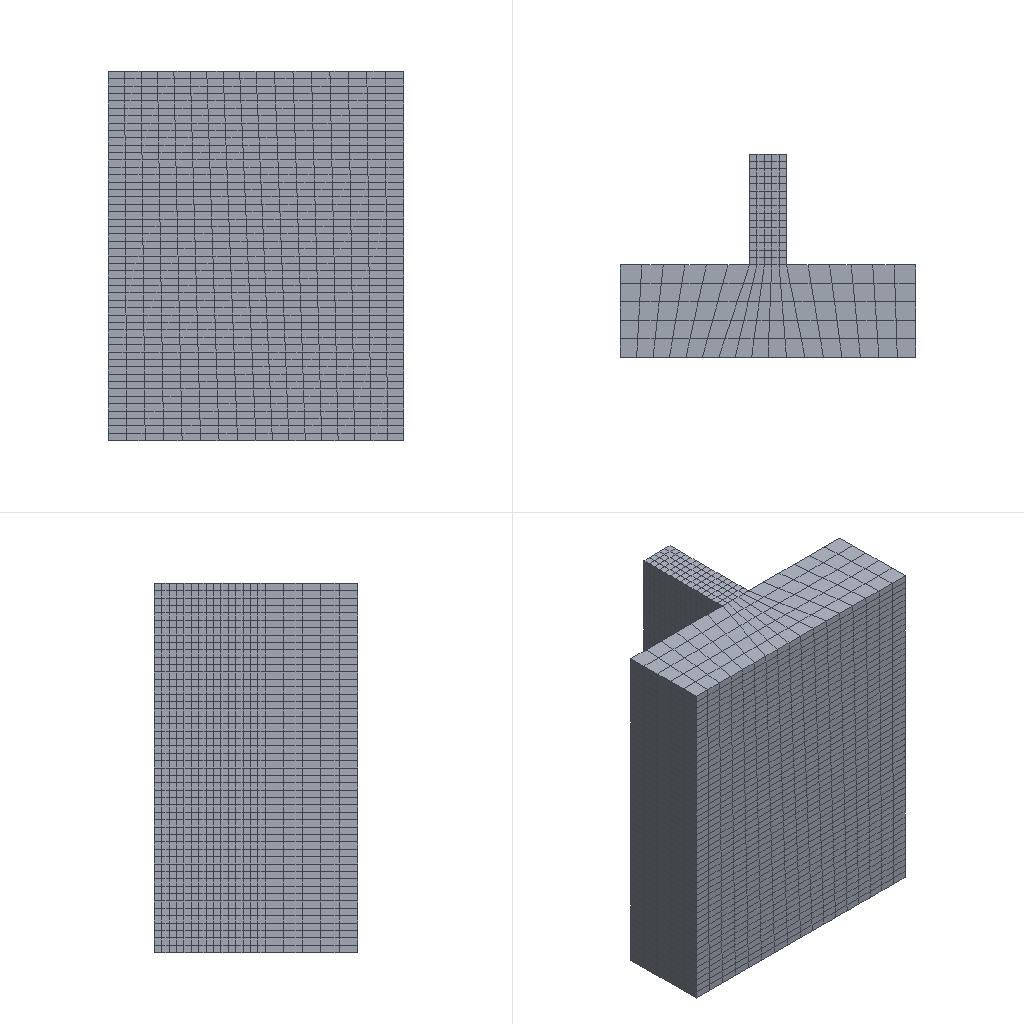Simulation study | abaqus
Set-up summary:
category,name,step,type,value,unit,region
solver,abaqus
solver,version,,,Abaqus/Standard 3DEXPERIENCE R2017x
units,not stated in the deck,,not stated
analysis,deck,,thermal,thermal
load_step,Step-kill,Step-kill,thermal
load_step,add-1,add-1,thermal
load_step,add-2,add-2,thermal
load_step,add-3,add-3,thermal
load_step,add-4,add-4,thermal
load_step,add-5,add-5,thermal
load_step,add-6,add-6,thermal
load_step,add-7,add-7,thermal
load_step,add-8,add-8,thermal
load_step,add-9,add-9,thermal
load_step,add-10,add-10,thermal
load_step,add-11,add-11,thermal
load_step,add-12,add-12,thermal
load_step,add-13,add-13,thermal
load_step,add-14,add-14,thermal
load_step,add-15,add-15,thermal
load_step,add-16,add-16,thermal
load_step,add-17,add-17,thermal
load_step,add-18,add-18,thermal
load_step,add-19,add-19,thermal
load_step,add-20,add-20,thermal
load_step,add-21,add-21,thermal
load_step,add-22,add-22,thermal
load_step,add-23,add-23,thermal
load_step,add-24,add-24,thermal
load_step,add-25,add-25,thermal
load_step,add-26,add-26,thermal
load_step,add-27,add-27,thermal
load_step,add-28,add-28,thermal
load_step,add-29,add-29,thermal
load_step,add-30,add-30,thermal
load_step,requested,,,31
mesh,nodes,,,10098
mesh,elements,,,8000
element_type,DC3D8,,solid,8000
load,load commands in deck,,count,4
bc,support commands in deck,,count,3
material,MATERIAL-1,,in results
check,setup vs results,,match,"per instance, exact: element labels, types and connectivity; labels of the nodes the elements use; coordinates of those nodes at SINGLE_PRECISION in 1 of 1 instance(s)"
Abaqus input file, long lists of numbers shortened:
*Heading
** Job name: Job-4 Model name: Model-1
** Generated by: Abaqus/CAE 2017
*Preprint, echo=NO, model=NO, history=NO, contact=NO
**
** PARTS
**
*Part, name=Part-1
*Node
      1,           5.,          10.,           0.
      2,           5.,          10.,         100.
** (10096 more lines like these left out)
*Element, type=DC3D8
   1,  246, 1185, 4611, 1153,    1,   27,  761,  132
   2, 1185, 1186, 4612, 4611,   27,   28,  762,  761
** (7998 more lines like these left out)
*Nset, nset=Set-4, generate
     1,  10098,      1
*Elset, elset=Set-4, generate
    1,  8000,     1
** Section: Section-1
*Solid Section, elset=Set-4, material=Material-1
,
*End Part
**
**
** ASSEMBLY
**
*Assembly, name=Assembly
**
*Instance, name=Part-1-1, part=Part-1
*End Instance
**
*Nset, nset=Set-1, instance=Part-1-1
    1,    2,    3,    4,    5,    6,    7,    8,    9,   10,   11,   12,   13,   14,   15,   16
   27,   28,   29,   30,   31,   32,   33,   34,   35,   36,   37,   38,   39,   40,   41,   42
** (304 more lines like these left out)
*Elset, elset=Set-1, instance=Part-1-1, generate
    1,  3750,     1
*Nset, nset=Set-2, instance=Part-1-1, generate
     1,  10098,      1
*Elset, elset=Set-2, instance=Part-1-1, generate
    1,  8000,     1
*Nset, nset=Set-3, instance=Part-1-1, generate
     1,  10098,      1
*Elset, elset=Set-3, instance=Part-1-1, generate
    1,  8000,     1
*Nset, nset=Set-36, instance=Part-1-1
    1,    2,    3,    4,    5,    6,    7,    8,    9,   10,   11,   12,   13,   14,   15,   16
   27,   28,   29,   30,   31,   32,   33,   34,   35,   36,   37,   38,   39,   40,   41,   42
** (304 more lines like these left out)
*Elset, elset=Set-36, instance=Part-1-1, generate
    1,  3750,     1
*Elset, elset=_PickedSet35, internal, instance=Part-1-1
    1,    2,    3,    4,    5,   51,   52,   53,   54,   55,  101,  102,  103,  104,  105,  151
  152,  153,  154,  155,  201,  202,  203,  204,  205,  251,  252,  253,  254,  255,  301,  302
** (6 more lines like these left out)
*Elset, elset=_PickedSet62, internal, instance=Part-1-1
    1,    2,    3,    4,    5,   51,   52,   53,   54,   55,  101,  102,  103,  104,  105,  151
  152,  153,  154,  155,  201,  202,  203,  204,  205,  251,  252,  253,  254,  255,  301,  302
** (6 more lines like these left out)
*Elset, elset=_PickedSet91, internal, instance=Part-1-1
    1,    2,    3,    4,    5,   51,   52,   53,   54,   55,  101,  102,  103,  104,  105,  151
  152,  153,  154,  155,  201,  202,  203,  204,  205,  251,  252,  253,  254,  255,  301,  302
** (6 more lines like these left out)
*Elset, elset=_PickedSet92, internal, instance=Part-1-1
    6,    7,    8,    9,   10,   56,   57,   58,   59,   60,  106,  107,  108,  109,  110,  156
  157,  158,  159,  160,  206,  207,  208,  209,  210,  256,  257,  258,  259,  260,  306,  307
** (6 more lines like these left out)
*Elset, elset=_PickedSet93, internal, instance=Part-1-1
   11,   12,   13,   14,   15,   61,   62,   63,   64,   65,  111,  112,  113,  114,  115,  161
  162,  163,  164,  165,  211,  212,  213,  214,  215,  261,  262,  263,  264,  265,  311,  312
** (6 more lines like these left out)
*Elset, elset=_PickedSet94, internal, instance=Part-1-1
   16,   17,   18,   19,   20,   66,   67,   68,   69,   70,  116,  117,  118,  119,  120,  166
  167,  168,  169,  170,  216,  217,  218,  219,  220,  266,  267,  268,  269,  270,  316,  317
** (6 more lines like these left out)
*Elset, elset=_PickedSet95, internal, instance=Part-1-1
   21,   22,   23,   24,   25,   71,   72,   73,   74,   75,  121,  122,  123,  124,  125,  171
  172,  173,  174,  175,  221,  222,  223,  224,  225,  271,  272,  273,  274,  275,  321,  322
** (6 more lines like these left out)
*Elset, elset=_PickedSet96, internal, instance=Part-1-1
   26,   27,   28,   29,   30,   76,   77,   78,   79,   80,  126,  127,  128,  129,  130,  176
  177,  178,  179,  180,  226,  227,  228,  229,  230,  276,  277,  278,  279,  280,  326,  327
** (6 more lines like these left out)
*Elset, elset=_PickedSet97, internal, instance=Part-1-1
   31,   32,   33,   34,   35,   81,   82,   83,   84,   85,  131,  132,  133,  134,  135,  181
  182,  183,  184,  185,  231,  232,  233,  234,  235,  281,  282,  283,  284,  285,  331,  332
** (6 more lines like these left out)
*Elset, elset=_PickedSet98, internal, instance=Part-1-1
   36,   37,   38,   39,   40,   86,   87,   88,   89,   90,  136,  137,  138,  139,  140,  186
  187,  188,  189,  190,  236,  237,  238,  239,  240,  286,  287,  288,  289,  290,  336,  337
** (6 more lines like these left out)
*Elset, elset=_PickedSet99, internal, instance=Part-1-1
   41,   42,   43,   44,   45,   91,   92,   93,   94,   95,  141,  142,  143,  144,  145,  191
  192,  193,  194,  195,  241,  242,  243,  244,  245,  291,  292,  293,  294,  295,  341,  342
** (6 more lines like these left out)
*Elset, elset=_PickedSet100, internal, instance=Part-1-1
   46,   47,   48,   49,   50,   96,   97,   98,   99,  100,  146,  147,  148,  149,  150,  196
  197,  198,  199,  200,  246,  247,  248,  249,  250,  296,  297,  298,  299,  300,  346,  347
** (6 more lines like these left out)
*Elset, elset=_PickedSet101, internal, instance=Part-1-1
 1296, 1297, 1298, 1299, 1300, 1346, 1347, 1348, 1349, 1350, 1396, 1397, 1398, 1399, 1400, 1446
 1447, 1448, 1449, 1450, 1496, 1497, 1498, 1499, 1500, 1546, 1547, 1548, 1549, 1550, 1596, 1597
** (6 more lines like these left out)
*Elset, elset=_PickedSet102, internal, instance=Part-1-1
 1291, 1292, 1293, 1294, 1295, 1341, 1342, 1343, 1344, 1345, 1391, 1392, 1393, 1394, 1395, 1441
 1442, 1443, 1444, 1445, 1491, 1492, 1493, 1494, 1495, 1541, 1542, 1543, 1544, 1545, 1591, 1592
** (6 more lines like these left out)
*Elset, elset=_PickedSet103, internal, instance=Part-1-1
 1286, 1287, 1288, 1289, 1290, 1336, 1337, 1338, 1339, 1340, 1386, 1387, 1388, 1389, 1390, 1436
 1437, 1438, 1439, 1440, 1486, 1487, 1488, 1489, 1490, 1536, 1537, 1538, 1539, 1540, 1586, 1587
** (6 more lines like these left out)
*Elset, elset=_PickedSet104, internal, instance=Part-1-1
 1281, 1282, 1283, 1284, 1285, 1331, 1332, 1333, 1334, 1335, 1381, 1382, 1383, 1384, 1385, 1431
 1432, 1433, 1434, 1435, 1481, 1482, 1483, 1484, 1485, 1531, 1532, 1533, 1534, 1535, 1581, 1582
** (6 more lines like these left out)
*Elset, elset=_PickedSet105, internal, instance=Part-1-1
 1276, 1277, 1278, 1279, 1280, 1326, 1327, 1328, 1329, 1330, 1376, 1377, 1378, 1379, 1380, 1426
 1427, 1428, 1429, 1430, 1476, 1477, 1478, 1479, 1480, 1526, 1527, 1528, 1529, 1530, 1576, 1577
** (6 more lines like these left out)
*Elset, elset=_PickedSet106, internal, instance=Part-1-1
 1271, 1272, 1273, 1274, 1275, 1321, 1322, 1323, 1324, 1325, 1371, 1372, 1373, 1374, 1375, 1421
 1422, 1423, 1424, 1425, 1471, 1472, 1473, 1474, 1475, 1521, 1522, 1523, 1524, 1525, 1571, 1572
** (6 more lines like these left out)
*Elset, elset=_PickedSet107, internal, instance=Part-1-1
 1266, 1267, 1268, 1269, 1270, 1316, 1317, 1318, 1319, 1320, 1366, 1367, 1368, 1369, 1370, 1416
 1417, 1418, 1419, 1420, 1466, 1467, 1468, 1469, 1470, 1516, 1517, 1518, 1519, 1520, 1566, 1567
** (6 more lines like these left out)
*Elset, elset=_PickedSet108, internal, instance=Part-1-1
 1261, 1262, 1263, 1264, 1265, 1311, 1312, 1313, 1314, 1315, 1361, 1362, 1363, 1364, 1365, 1411
 1412, 1413, 1414, 1415, 1461, 1462, 1463, 1464, 1465, 1511, 1512, 1513, 1514, 1515, 1561, 1562
** (6 more lines like these left out)
*Elset, elset=_PickedSet109, internal, instance=Part-1-1
 1256, 1257, 1258, 1259, 1260, 1306, 1307, 1308, 1309, 1310, 1356, 1357, 1358, 1359, 1360, 1406
 1407, 1408, 1409, 1410, 1456, 1457, 1458, 1459, 1460, 1506, 1507, 1508, 1509, 1510, 1556, 1557
** (6 more lines like these left out)
*Elset, elset=_PickedSet110, internal, instance=Part-1-1
 1251, 1252, 1253, 1254, 1255, 1301, 1302, 1303, 1304, 1305, 1351, 1352, 1353, 1354, 1355, 1401
 1402, 1403, 1404, 1405, 1451, 1452, 1453, 1454, 1455, 1501, 1502, 1503, 1504, 1505, 1551, 1552
** (6 more lines like these left out)
*Elset, elset=_PickedSet111, internal, instance=Part-1-1
 2501, 2502, 2503, 2504, 2505, 2551, 2552, 2553, 2554, 2555, 2601, 2602, 2603, 2604, 2605, 2651
 2652, 2653, 2654, 2655, 2701, 2702, 2703, 2704, 2705, 2751, 2752, 2753, 2754, 2755, 2801, 2802
** (6 more lines like these left out)
*Elset, elset=_PickedSet112, internal, instance=Part-1-1
 2506, 2507, 2508, 2509, 2510, 2556, 2557, 2558, 2559, 2560, 2606, 2607, 2608, 2609, 2610, 2656
 2657, 2658, 2659, 2660, 2706, 2707, 2708, 2709, 2710, 2756, 2757, 2758, 2759, 2760, 2806, 2807
** (6 more lines like these left out)
*Elset, elset=_PickedSet113, internal, instance=Part-1-1
 2511, 2512, 2513, 2514, 2515, 2561, 2562, 2563, 2564, 2565, 2611, 2612, 2613, 2614, 2615, 2661
 2662, 2663, 2664, 2665, 2711, 2712, 2713, 2714, 2715, 2761, 2762, 2763, 2764, 2765, 2811, 2812
** (6 more lines like these left out)
*Elset, elset=_PickedSet114, internal, instance=Part-1-1
 2516, 2517, 2518, 2519, 2520, 2566, 2567, 2568, 2569, 2570, 2616, 2617, 2618, 2619, 2620, 2666
 2667, 2668, 2669, 2670, 2716, 2717, 2718, 2719, 2720, 2766, 2767, 2768, 2769, 2770, 2816, 2817
** (6 more lines like these left out)
*Elset, elset=_PickedSet115, internal, instance=Part-1-1
 2521, 2522, 2523, 2524, 2525, 2571, 2572, 2573, 2574, 2575, 2621, 2622, 2623, 2624, 2625, 2671
 2672, 2673, 2674, 2675, 2721, 2722, 2723, 2724, 2725, 2771, 2772, 2773, 2774, 2775, 2821, 2822
** (6 more lines like these left out)
*Elset, elset=_PickedSet116, internal, instance=Part-1-1
 2526, 2527, 2528, 2529, 2530, 2576, 2577, 2578, 2579, 2580, 2626, 2627, 2628, 2629, 2630, 2676
 2677, 2678, 2679, 2680, 2726, 2727, 2728, 2729, 2730, 2776, 2777, 2778, 2779, 2780, 2826, 2827
** (6 more lines like these left out)
*Elset, elset=_PickedSet117, internal, instance=Part-1-1
 2531, 2532, 2533, 2534, 2535, 2581, 2582, 2583, 2584, 2585, 2631, 2632, 2633, 2634, 2635, 2681
 2682, 2683, 2684, 2685, 2731, 2732, 2733, 2734, 2735, 2781, 2782, 2783, 2784, 2785, 2831, 2832
** (6 more lines like these left out)
*Elset, elset=_PickedSet118, internal, instance=Part-1-1
 2536, 2537, 2538, 2539, 2540, 2586, 2587, 2588, 2589, 2590, 2636, 2637, 2638, 2639, 2640, 2686
 2687, 2688, 2689, 2690, 2736, 2737, 2738, 2739, 2740, 2786, 2787, 2788, 2789, 2790, 2836, 2837
** (6 more lines like these left out)
*Elset, elset=_PickedSet119, internal, instance=Part-1-1
 2541, 2542, 2543, 2544, 2545, 2591, 2592, 2593, 2594, 2595, 2641, 2642, 2643, 2644, 2645, 2691
 2692, 2693, 2694, 2695, 2741, 2742, 2743, 2744, 2745, 2791, 2792, 2793, 2794, 2795, 2841, 2842
** (6 more lines like these left out)
*Elset, elset=_PickedSet120, internal, instance=Part-1-1
 2546, 2547, 2548, 2549, 2550, 2596, 2597, 2598, 2599, 2600, 2646, 2647, 2648, 2649, 2650, 2696
 2697, 2698, 2699, 2700, 2746, 2747, 2748, 2749, 2750, 2796, 2797, 2798, 2799, 2800, 2846, 2847
** (6 more lines like these left out)
*Elset, elset=_Surf-1_S4, internal, instance=Part-1-1, generate
   50,  8000,    50
*Elset, elset=_Surf-1_S6, internal, instance=Part-1-1, generate
    1,  7951,    50
*Elset, elset=_Surf-1_S1, internal, instance=Part-1-1
 1001, 1002, 1003, 1004, 1005, 1006, 1007, 1008, 1009, 1010, 1011, 1012, 1013, 1014, 1015, 1016
 1017, 1018, 1019, 1020, 1021, 1022, 1023, 1024, 1025, 1026, 1027, 1028, 1029, 1030, 1031, 1032
** (83 more lines like these left out)
*Elset, elset=_Surf-1_S2, internal, instance=Part-1-1
    1,    2,    3,    4,    5,    6,    7,    8,    9,   10,   11,   12,   13,   14,   15,   16
   17,   18,   19,   20,   21,   22,   23,   24,   25,   26,   27,   28,   29,   30,   31,   32
** (98 more lines like these left out)
*Elset, elset=_Surf-1_S5, internal, instance=Part-1-1
 2701, 2702, 2703, 2704, 2705, 2706, 2707, 2708, 2709, 2710, 2711, 2712, 2713, 2714, 2715, 2716
 2717, 2718, 2719, 2720, 2721, 2722, 2723, 2724, 2725, 2726, 2727, 2728, 2729, 2730, 2731, 2732
** (30 more lines like these left out)
*Elset, elset=_Surf-1_S3, internal, instance=Part-1-1
 3751, 3752, 3753, 3754, 3755, 3756, 3757, 3758, 3759, 3760, 3761, 3762, 3763, 3764, 3765, 3766
 3767, 3768, 3769, 3770, 3771, 3772, 3773, 3774, 3775, 3776, 3777, 3778, 3779, 3780, 3781, 3782
** (14 more lines like these left out)
*Surface, type=ELEMENT, name=Surf-1
_Surf-1_S4, S4
_Surf-1_S6, S6
_Surf-1_S2, S2
_Surf-1_S1, S1
_Surf-1_S5, S5
_Surf-1_S3, S3
*Elset, elset=_Surf-2_S4, internal, instance=Part-1-1, generate
   50,  8000,    50
*Elset, elset=_Surf-2_S6, internal, instance=Part-1-1, generate
    1,  7951,    50
*Elset, elset=_Surf-2_S1, internal, instance=Part-1-1
 1001, 1002, 1003, 1004, 1005, 1006, 1007, 1008, 1009, 1010, 1011, 1012, 1013, 1014, 1015, 1016
 1017, 1018, 1019, 1020, 1021, 1022, 1023, 1024, 1025, 1026, 1027, 1028, 1029, 1030, 1031, 1032
** (83 more lines like these left out)
*Elset, elset=_Surf-2_S2, internal, instance=Part-1-1
    1,    2,    3,    4,    5,    6,    7,    8,    9,   10,   11,   12,   13,   14,   15,   16
   17,   18,   19,   20,   21,   22,   23,   24,   25,   26,   27,   28,   29,   30,   31,   32
** (98 more lines like these left out)
*Elset, elset=_Surf-2_S5, internal, instance=Part-1-1
 2701, 2702, 2703, 2704, 2705, 2706, 2707, 2708, 2709, 2710, 2711, 2712, 2713, 2714, 2715, 2716
 2717, 2718, 2719, 2720, 2721, 2722, 2723, 2724, 2725, 2726, 2727, 2728, 2729, 2730, 2731, 2732
** (30 more lines like these left out)
*Elset, elset=_Surf-2_S3, internal, instance=Part-1-1
 3751, 3752, 3753, 3754, 3755, 3756, 3757, 3758, 3759, 3760, 3761, 3762, 3763, 3764, 3765, 3766
 3767, 3768, 3769, 3770, 3771, 3772, 3773, 3774, 3775, 3776, 3777, 3778, 3779, 3780, 3781, 3782
** (14 more lines like these left out)
*Surface, type=ELEMENT, name=Surf-2
_Surf-2_S4, S4
_Surf-2_S6, S6
_Surf-2_S2, S2
_Surf-2_S1, S1
_Surf-2_S5, S5
_Surf-2_S3, S3
*End Assembly
**
** MATERIALS
**
*Material, name=Material-1
*Conductivity
134.,
*Density
 2.2e-09,
*Elastic
72000., 0.35
*Expansion
 2.32e-05,
*Specific Heat
 8.6e+08,
**
** PHYSICAL CONSTANTS
**
*Physical Constants, absolute zero=-273., stefan boltzmann=5.67e-08
**
** PREDEFINED FIELDS
**
** Name: Predefined Field-1   Type: Temperature
*Initial Conditions, type=TEMPERATURE
Set-3, 25.
** ----------------------------------------------------------------
**
** STEP: Step-kill
**
*Step, name=Step-kill, nlgeom=NO
*Heat Transfer, end=PERIOD, deltmx=1000., mxdem=1.
0.0001, 0.0001, 1e-09, 0.0001,
**
** INTERACTIONS
**
** Interaction: kill-all
*Model Change, remove
Set-36,
**
** OUTPUT REQUESTS
**
*Restart, write, frequency=0
**
** FIELD OUTPUT: F-Output-1
**
*Output, field
*Node Output
NT, RFL
*Element Output, directions=YES
HFL, TEMP
*Output, history, frequency=0
*End Step
** ----------------------------------------------------------------
**
** STEP: add-1
**
*Step, name=add-1, nlgeom=NO, inc=10000
*Heat Transfer, end=PERIOD, deltmx=10000., mxdem=1.
0.1, 1., 1e-05, 1.,
**
** LOADS
**
** Name: Load-1   Type: Body heat flux
*Dflux
Set-2, BFNU, 1.
**
** INTERACTIONS
**
** Interaction: add-1
*Model Change, add
_PickedSet91,
** Interaction: heat-translate
*Sfilm
Surf-1, F, 25., 0.05
** Interaction: heat-translate2
*Sradiate
Surf-2, R, 25., 0.5
**
** OUTPUT REQUESTS
**
*Restart, write, frequency=0
**
** FIELD OUTPUT: F-Output-1
**
*Output, field
*Node Output
NT, RFL
*Element Output, directions=YES
HFL, TEMP
*Output, history, frequency=0
*End Step
** ----------------------------------------------------------------
**
** STEP: add-2
**
*Step, name=add-2, nlgeom=NO, inc=1000000
*Heat Transfer, end=PERIOD, deltmx=1000.
0.05, 1., 1e-11, 0.2,
**
** INTERACTIONS
**
** Interaction: add-2
*Model Change, add
_PickedSet92,
**
** OUTPUT REQUESTS
**
*Restart, write, frequency=0
**
** FIELD OUTPUT: F-Output-1
**
*Output, field
*Node Output
NT, RFL
*Element Output, directions=YES
HFL, TEMP
*Output, history, frequency=0
*End Step
** ----------------------------------------------------------------
**
** STEP: add-3
**
*Step, name=add-3, nlgeom=NO, inc=1000000
*Heat Transfer, end=PERIOD, deltmx=1000.
0.05, 1., 1e-11, 0.2,
**
** INTERACTIONS
**
** Interaction: add-3
*Model Change, add
_PickedSet93,
**
** OUTPUT REQUESTS
**
*Restart, write, frequency=0
**
** FIELD OUTPUT: F-Output-1
**
*Output, field
*Node Output
NT, RFL
*Element Output, directions=YES
HFL, TEMP
*Output, history, frequency=0
*End Step
** ----------------------------------------------------------------
**
** STEP: add-4
**
*Step, name=add-4, nlgeom=NO, inc=1000000
*Heat Transfer, end=PERIOD, deltmx=1000.
0.05, 1., 1e-11, 0.2,
**
** INTERACTIONS
**
** Interaction: add-4
*Model Change, add
_PickedSet94,
**
** OUTPUT REQUESTS
**
*Restart, write, frequency=0
**
** FIELD OUTPUT: F-Output-1
**
*Output, field
*Node Output
NT, RFL
*Element Output, directions=YES
HFL, TEMP
*Output, history, frequency=0
*End Step
** ----------------------------------------------------------------
**
** STEP: add-5
**
*Step, name=add-5, nlgeom=NO, inc=1000000
*Heat Transfer, end=PERIOD, deltmx=1000.
0.05, 1., 1e-11, 0.2,
**
** INTERACTIONS
**
** Interaction: add-5
*Model Change, add
_PickedSet95,
**
** OUTPUT REQUESTS
**
*Restart, write, frequency=0
**
** FIELD OUTPUT: F-Output-1
**
*Output, field
*Node Output
NT, RFL
*Element Output, directions=YES
HFL, TEMP
*Output, history, frequency=0
*End Step
** ----------------------------------------------------------------
**
** STEP: add-6
**
*Step, name=add-6, nlgeom=NO, inc=1000000
*Heat Transfer, end=PERIOD, deltmx=1000.
0.05, 1., 1e-11, 0.2,
**
** INTERACTIONS
**
** Interaction: add-6
*Model Change, add
_PickedSet96,
**
** OUTPUT REQUESTS
**
*Restart, write, frequency=0
**
** FIELD OUTPUT: F-Output-1
**
*Output, field
*Node Output
NT, RFL
*Element Output, directions=YES
HFL, TEMP
*Output, history, frequency=0
*End Step
** ----------------------------------------------------------------
**
** STEP: add-7
**
*Step, name=add-7, nlgeom=NO, inc=1000000
*Heat Transfer, end=PERIOD, deltmx=1000.
0.05, 1., 1e-11, 0.2,
**
** INTERACTIONS
**
** Interaction: add-7
*Model Change, add
_PickedSet97,
**
** OUTPUT REQUESTS
**
*Restart, write, frequency=0
**
** FIELD OUTPUT: F-Output-1
**
*Output, field
*Node Output
NT, RFL
*Element Output, directions=YES
HFL, TEMP
*Output, history, frequency=0
*End Step
** ----------------------------------------------------------------
**
** STEP: add-8
**
*Step, name=add-8, nlgeom=NO, inc=1000000
*Heat Transfer, end=PERIOD, deltmx=1000.
0.05, 1., 1e-11, 0.2,
**
** INTERACTIONS
**
** Interaction: add-8
*Model Change, add
_PickedSet98,
**
** OUTPUT REQUESTS
**
*Restart, write, frequency=0
**
** FIELD OUTPUT: F-Output-1
**
*Output, field
*Node Output
NT, RFL
*Element Output, directions=YES
HFL, TEMP
*Output, history, frequency=0
*End Step
** ----------------------------------------------------------------
**
** STEP: add-9
**
*Step, name=add-9, nlgeom=NO, inc=1000000
*Heat Transfer, end=PERIOD, deltmx=1000.
0.05, 1., 1e-11, 0.2,
**
** INTERACTIONS
**
** Interaction: add-9
*Model Change, add
_PickedSet99,
**
** OUTPUT REQUESTS
**
*Restart, write, frequency=0
**
** FIELD OUTPUT: F-Output-1
**
*Output, field
*Node Output
NT, RFL
*Element Output, directions=YES
HFL, TEMP
*Output, history, frequency=0
*End Step
** ----------------------------------------------------------------
**
** STEP: add-10
**
*Step, name=add-10, nlgeom=NO, inc=1000000
*Heat Transfer, end=PERIOD, deltmx=1000.
0.05, 1., 1e-11, 0.2,
**
** INTERACTIONS
**
** Interaction: add-10
*Model Change, add
_PickedSet100,
**
** OUTPUT REQUESTS
**
*Restart, write, frequency=0
**
** FIELD OUTPUT: F-Output-1
**
*Output, field
*Node Output
NT, RFL
*Element Output, directions=YES
HFL, TEMP
*Output, history, frequency=0
*End Step
** ----------------------------------------------------------------
**
** STEP: add-11
**
*Step, name=add-11, nlgeom=NO, inc=1000000
*Heat Transfer, end=PERIOD, deltmx=1000.
0.05, 1., 1e-11, 0.2,
**
** INTERACTIONS
**
** Interaction: add-11
*Model Change, add
_PickedSet101,
** Interaction: heat-translate
*Sfilm
Surf-1, F, 25., 0.6
**
** OUTPUT REQUESTS
**
*Restart, write, frequency=0
**
** FIELD OUTPUT: F-Output-1
**
*Output, field
*Node Output
NT, RFL
*Element Output, directions=YES
HFL, TEMP
*Output, history, frequency=0
*End Step
** ----------------------------------------------------------------
**
** STEP: add-12
**
*Step, name=add-12, nlgeom=NO, inc=1000000
*Heat Transfer, end=PERIOD, deltmx=1000.
0.05, 1., 1e-11, 0.2,
**
** INTERACTIONS
**
** Interaction: add-12
*Model Change, add
_PickedSet102,
**
** OUTPUT REQUESTS
**
*Restart, write, frequency=0
**
** FIELD OUTPUT: F-Output-1
**
*Output, field
*Node Output
NT, RFL
*Element Output, directions=YES
HFL, TEMP
*Output, history, frequency=0
*End Step
** ----------------------------------------------------------------
**
** STEP: add-13
**
*Step, name=add-13, nlgeom=NO, inc=1000000
*Heat Transfer, end=PERIOD, deltmx=1000.
0.05, 1., 1e-11, 0.2,
**
** INTERACTIONS
**
** Interaction: add-13
*Model Change, add
_PickedSet103,
**
** OUTPUT REQUESTS
**
*Restart, write, frequency=0
**
** FIELD OUTPUT: F-Output-1
**
*Output, field
*Node Output
NT, RFL
*Element Output, directions=YES
HFL, TEMP
*Output, history, frequency=0
*End Step
** ----------------------------------------------------------------
**
** STEP: add-14
**
*Step, name=add-14, nlgeom=NO, inc=1000000
*Heat Transfer, end=PERIOD, deltmx=1000.
0.05, 1., 1e-11, 0.2,
**
** INTERACTIONS
**
** Interaction: add-14
*Model Change, add
_PickedSet104,
**
** OUTPUT REQUESTS
**
*Restart, write, frequency=0
**
** FIELD OUTPUT: F-Output-1
**
*Output, field
*Node Output
NT, RFL
*Element Output, directions=YES
HFL, TEMP
*Output, history, frequency=0
*End Step
** ----------------------------------------------------------------
**
** STEP: add-15
**
*Step, name=add-15, nlgeom=NO, inc=1000000
*Heat Transfer, end=PERIOD, deltmx=1000.
0.05, 1., 1e-11, 0.2,
**
** INTERACTIONS
**
** Interaction: add-15
*Model Change, add
_PickedSet105,
**
** OUTPUT REQUESTS
**
*Restart, write, frequency=0
**
** FIELD OUTPUT: F-Output-1
**
*Output, field
*Node Output
NT, RFL
*Element Output, directions=YES
HFL, TEMP
*Output, history, frequency=0
*End Step
** ----------------------------------------------------------------
**
** STEP: add-16
**
*Step, name=add-16, nlgeom=NO, inc=1000000
*Heat Transfer, end=PERIOD, deltmx=1000.
0.05, 1., 1e-11, 0.2,
**
** INTERACTIONS
**
** Interaction: add-16
*Model Change, add
_PickedSet106,
**
** OUTPUT REQUESTS
**
*Restart, write, frequency=0
**
** FIELD OUTPUT: F-Output-1
**
*Output, field
*Node Output
NT, RFL
*Element Output, directions=YES
HFL, TEMP
*Output, history, frequency=0
*End Step
** ----------------------------------------------------------------
**
** STEP: add-17
**
*Step, name=add-17, nlgeom=NO, inc=1000000
*Heat Transfer, end=PERIOD, deltmx=1000.
0.05, 1., 1e-11, 0.2,
**
** INTERACTIONS
**
** Interaction: add-17
*Model Change, add
_PickedSet107,
**
** OUTPUT REQUESTS
**
*Restart, write, frequency=0
**
** FIELD OUTPUT: F-Output-1
**
*Output, field
*Node Output
NT, RFL
*Element Output, directions=YES
HFL, TEMP
*Output, history, frequency=0
*End Step
** ----------------------------------------------------------------
**
** STEP: add-18
**
*Step, name=add-18, nlgeom=NO, inc=1000000
*Heat Transfer, end=PERIOD, deltmx=1000.
0.05, 1., 1e-11, 0.2,
**
** INTERACTIONS
**
** Interaction: add-18
*Model Change, add
_PickedSet108,
**
** OUTPUT REQUESTS
**
*Restart, write, frequency=0
**
** FIELD OUTPUT: F-Output-1
**
*Output, field
*Node Output
NT, RFL
*Element Output, directions=YES
HFL, TEMP
*Output, history, frequency=0
*End Step
** ----------------------------------------------------------------
**
** STEP: add-19
**
*Step, name=add-19, nlgeom=NO, inc=1000000
*Heat Transfer, end=PERIOD, deltmx=1000.
0.05, 1., 1e-11, 0.2,
**
** INTERACTIONS
**
** Interaction: add-19
*Model Change, add
_PickedSet109,
**
** OUTPUT REQUESTS
**
*Restart, write, frequency=0
**
** FIELD OUTPUT: F-Output-1
**
*Output, field
*Node Output
NT, RFL
*Element Output, directions=YES
HFL, TEMP
*Output, history, frequency=0
*End Step
** ----------------------------------------------------------------
**
** STEP: add-20
**
*Step, name=add-20, nlgeom=NO, inc=1000000
*Heat Transfer, end=PERIOD, deltmx=1000.
0.05, 1., 1e-11, 0.2,
**
** INTERACTIONS
**
** Interaction: add-20
*Model Change, add
_PickedSet110,
**
** OUTPUT REQUESTS
**
*Restart, write, frequency=0
**
** FIELD OUTPUT: F-Output-1
**
*Output, field
*Node Output
NT, RFL
*Element Output, directions=YES
HFL, TEMP
*Output, history, frequency=0
*End Step
** ----------------------------------------------------------------
**
** STEP: add-21
**
*Step, name=add-21, nlgeom=NO, inc=1000000
*Heat Transfer, end=PERIOD, deltmx=1000.
0.05, 1., 1e-11, 0.2,
**
** INTERACTIONS
**
** Interaction: add-21
*Model Change, add
_PickedSet111,
**
** OUTPUT REQUESTS
**
*Restart, write, frequency=0
**
** FIELD OUTPUT: F-Output-1
**
*Output, field
*Node Output
NT, RFL
*Element Output, directions=YES
HFL, TEMP
*Output, history, frequency=0
*End Step
** ----------------------------------------------------------------
**
** STEP: add-22
**
*Step, name=add-22, nlgeom=NO, inc=1000000
*Heat Transfer, end=PERIOD, deltmx=1000.
0.05, 1., 1e-11, 0.2,
**
** INTERACTIONS
**
** Interaction: add-22
*Model Change, add
_PickedSet112,
**
** OUTPUT REQUESTS
**
*Restart, write, frequency=0
**
** FIELD OUTPUT: F-Output-1
**
*Output, field
*Node Output
NT, RFL
*Element Output, directions=YES
HFL, TEMP
*Output, history, frequency=0
*End Step
** ----------------------------------------------------------------
**
** STEP: add-23
**
*Step, name=add-23, nlgeom=NO, inc=1000000
*Heat Transfer, end=PERIOD, deltmx=1000.
0.05, 1., 1e-11, 0.2,
**
** INTERACTIONS
**
** Interaction: add-23
*Model Change, add
_PickedSet113,
**
** OUTPUT REQUESTS
**
*Restart, write, frequency=0
**
** FIELD OUTPUT: F-Output-1
**
*Output, field
*Node Output
NT, RFL
*Element Output, directions=YES
HFL, TEMP
*Output, history, frequency=0
*End Step
** ----------------------------------------------------------------
**
** STEP: add-24
**
*Step, name=add-24, nlgeom=NO, inc=1000000
*Heat Transfer, end=PERIOD, deltmx=1000.
0.05, 1., 1e-11, 0.2,
**
** INTERACTIONS
**
** Interaction: add-24
*Model Change, add
_PickedSet114,
**
** OUTPUT REQUESTS
**
*Restart, write, frequency=0
**
** FIELD OUTPUT: F-Output-1
**
*Output, field
*Node Output
NT, RFL
*Element Output, directions=YES
HFL, TEMP
*Output, history, frequency=0
*End Step
** ----------------------------------------------------------------
**
** STEP: add-25
**
*Step, name=add-25, nlgeom=NO, inc=1000000
*Heat Transfer, end=PERIOD, deltmx=1000.
0.05, 1., 1e-11, 0.2,
**
** INTERACTIONS
**
** Interaction: add-25
*Model Change, add
_PickedSet115,
**
** OUTPUT REQUESTS
**
*Restart, write, frequency=0
**
** FIELD OUTPUT: F-Output-1
**
*Output, field
*Node Output
NT, RFL
*Element Output, directions=YES
HFL, TEMP
*Output, history, frequency=0
*End Step
** ----------------------------------------------------------------
**
** STEP: add-26
**
*Step, name=add-26, nlgeom=NO, inc=1000000
*Heat Transfer, end=PERIOD, deltmx=1000.
0.05, 1., 1e-11, 0.2,
**
** INTERACTIONS
**
** Interaction: add-26
*Model Change, add
_PickedSet116,
**
** OUTPUT REQUESTS
**
*Restart, write, frequency=0
**
** FIELD OUTPUT: F-Output-1
**
*Output, field
*Node Output
NT, RFL
*Element Output, directions=YES
HFL, TEMP
*Output, history, frequency=0
*End Step
** ----------------------------------------------------------------
**
** STEP: add-27
**
*Step, name=add-27, nlgeom=NO, inc=1000000
*Heat Transfer, end=PERIOD, deltmx=1000.
0.05, 1., 1e-11, 0.2,
**
** INTERACTIONS
**
** Interaction: add-27
*Model Change, add
_PickedSet117,
**
** OUTPUT REQUESTS
**
*Restart, write, frequency=0
**
** FIELD OUTPUT: F-Output-1
**
*Output, field
*Node Output
NT, RFL
*Element Output, directions=YES
HFL, TEMP
*Output, history, frequency=0
*End Step
** ----------------------------------------------------------------
**
** STEP: add-28
**
*Step, name=add-28, nlgeom=NO, inc=1000000
*Heat Transfer, end=PERIOD, deltmx=1000.
0.05, 1., 1e-11, 0.2,
**
** INTERACTIONS
**
** Interaction: add-28
*Model Change, add
_PickedSet118,
**
** OUTPUT REQUESTS
**
*Restart, write, frequency=0
**
** FIELD OUTPUT: F-Output-1
**
*Output, field
*Node Output
NT, RFL
*Element Output, directions=YES
HFL, TEMP
*Output, history, frequency=0
*End Step
** ----------------------------------------------------------------
**
** STEP: add-29
**
*Step, name=add-29, nlgeom=NO, inc=1000000
*Heat Transfer, end=PERIOD, deltmx=1000.
0.05, 1., 1e-11, 0.2,
**
** INTERACTIONS
**
** Interaction: add-29
*Model Change, add
_PickedSet119,
**
** OUTPUT REQUESTS
**
*Restart, write, frequency=0
**
** FIELD OUTPUT: F-Output-1
**
*Output, field
*Node Output
NT, RFL
*Element Output, directions=YES
HFL, TEMP
*Output, history, frequency=0
*End Step
** ----------------------------------------------------------------
**
** STEP: add-30
**
*Step, name=add-30, nlgeom=NO, inc=1000000
*Heat Transfer, end=PERIOD, deltmx=1000.
0.05, 1., 1e-11, 0.2,
**
** INTERACTIONS
**
** Interaction: add-30
*Model Change, add
_PickedSet120,
**
** OUTPUT REQUESTS
**
*Restart, write, frequency=0
**
** FIELD OUTPUT: F-Output-1
**
*Output, field
*Node Output
NT, RFL
*Element Output, directions=YES
HFL, TEMP
*Output, history, frequency=0
*End Step
Results summary:
result,step,,partial,increments=0 time=0.0/0.0001
result,step,,partial,increments=0 time=0.0/1.0
result,step,,partial,increments=0 time=0.0/1.0
result,step,,partial,increments=0 time=0.0/1.0
result,step,,partial,increments=0 time=0.0/1.0
result,step,,partial,increments=0 time=0.0/1.0
result,step,,partial,increments=0 time=0.0/1.0
result,step,,partial,increments=0 time=0.0/1.0
result,step,,partial,increments=0 time=0.0/1.0
result,step,,partial,increments=0 time=0.0/1.0
result,step,,partial,increments=0 time=0.0/1.0
result,step,,partial,increments=0 time=0.0/1.0
result,step,,partial,increments=0 time=0.0/1.0
result,step,,partial,increments=0 time=0.0/1.0
result,step,,partial,increments=0 time=0.0/1.0
result,step,,partial,increments=0 time=0.0/1.0
result,step,,partial,increments=0 time=0.0/1.0
result,step,,partial,increments=0 time=0.0/1.0
result,step,,partial,increments=0 time=0.0/1.0
result,step,,partial,increments=0 time=0.0/1.0
result,step,,partial,increments=0 time=0.0/1.0
result,step,,partial,increments=0 time=0.0/1.0
result,step,,partial,increments=0 time=0.0/1.0
result,step,,partial,increments=0 time=0.0/1.0
result,step,,partial,increments=0 time=0.0/1.0
result,step,,partial,increments=0 time=0.0/1.0
result,step,,partial,increments=0 time=0.0/1.0
result,step,,partial,increments=0 time=0.0/1.0
result,step,,partial,increments=0 time=0.0/1.0
result,step,,partial,increments=0 time=0.0/1.0
result,step,,partial,increments=0 time=0.0/1.0
result,analysis,,,"heat transfer, deltamx"
result,last_loadstep,,,31
result,primary field,,,NT11